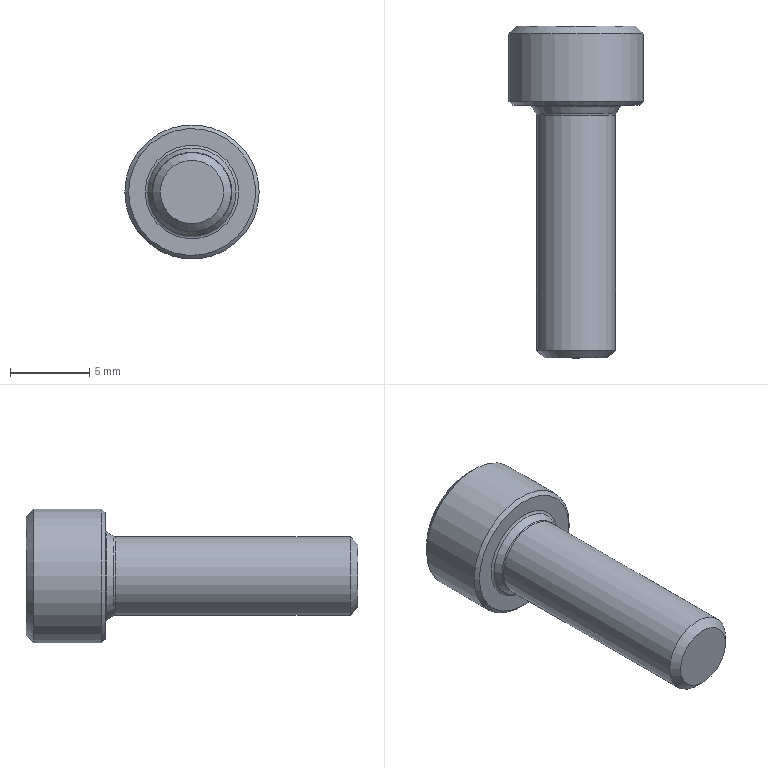Part | STEP file | 1 solid | 31 faces | box 8.5 x 21 x 8.5 mm | volume 546.765 mm3 | plane 15 | cone 11 | cylinder 3 | torus 2 | commonest cylinder face diameters 4 x1 5 x1 8.5 x1